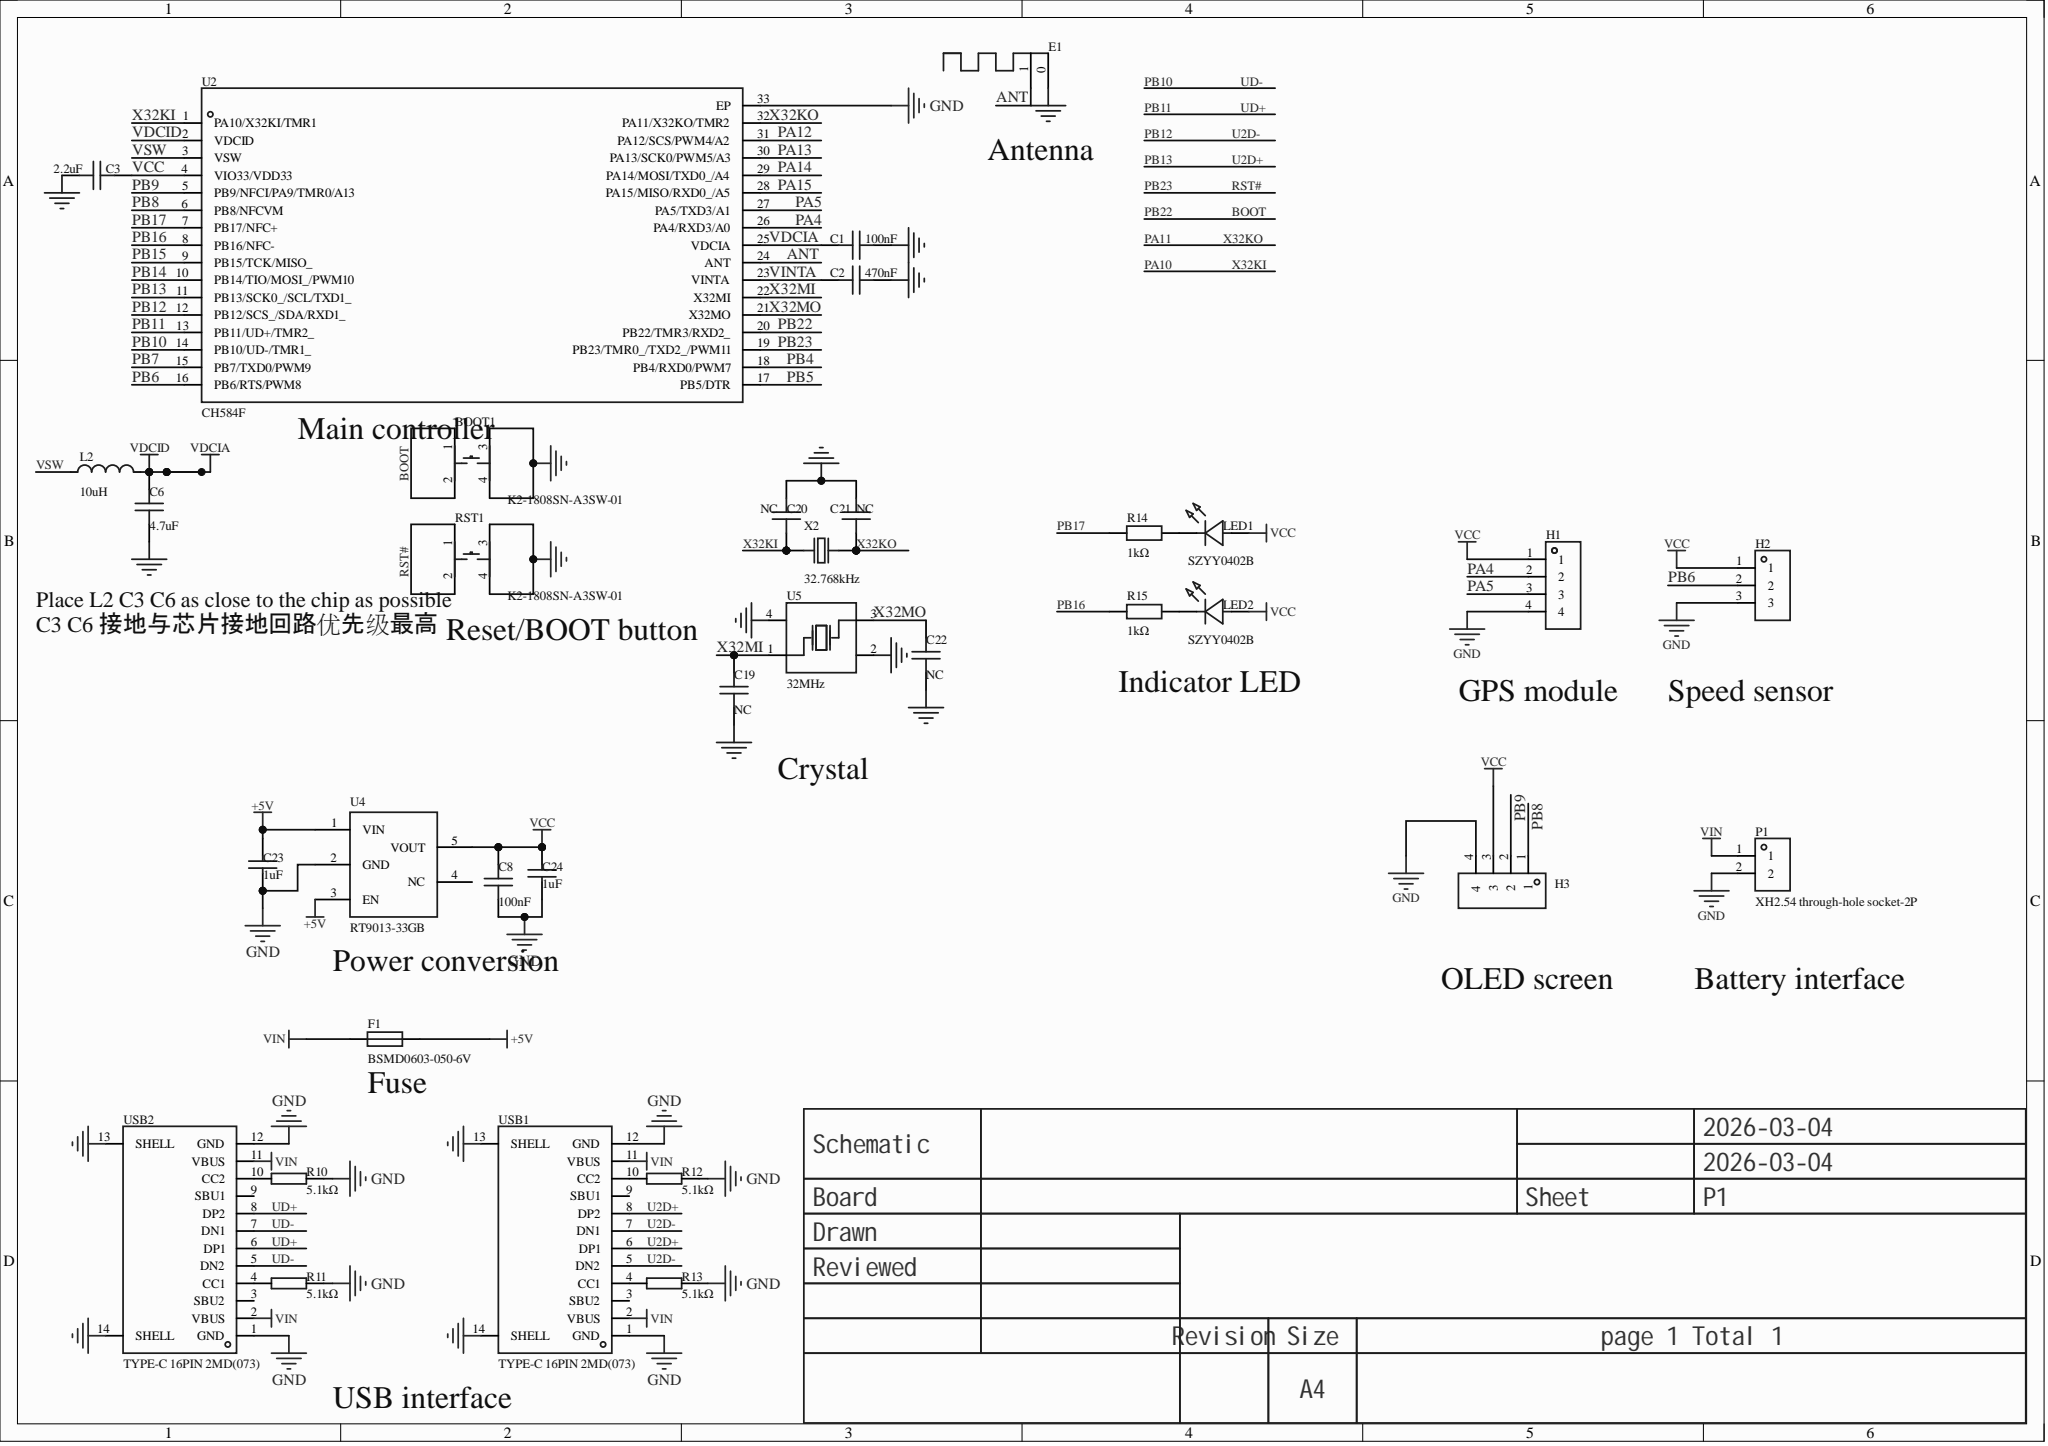Circuit board | Altium Designer | 34 parts | 31 nets
Bill of materials:
Comment,Description,Designator,Footprint,LibRef,Quantity
"K2-1808SN-A3SW-01","","BOOT1, RST1","SW-SMD_4P-L4.2-W3.3-P2.15-LS5.1","K2-1808SN-A3SW-01","2"
"100nF","[NoValue], Capacitance: 100nF; tolerance: ±10%; rated voltage: -; dielectric (temperature coefficient): -;","C1, C8","0402电容（极简封装）","CAP_0402, GCM155R71C104KA55J","2"
"470nF","","C2","0402电容（极简封装）","CAP_0402","1"
"2.2uF","","C3","0402电容（极简封装）","CAP_0402","1"
"4.7uF","","C6","0402电容（极简封装）","CAP_0402","1"
"NC","","C19, C20, C21, C22","0402电容（极简封装）","CAP_0402","4"
"1uF","Capacitance: 1uF; tolerance: ±10%; rated voltage: 16V; temperature coefficient: X5R;","C23, C24","0402电容（极简封装）","EMK105BJ105KV-F","2"
"","","E1","ANT-F-1-2.4G-1.6mmFR4","2.4G天线","1"
"BSMD0603-050-6V","Withstand voltage (Vmax): 6V; max current (Imax): 40A; hold current (Ihold): 500mA; trip current (Itrip): 1A;","F1","F0603","BSMD0603-050-6V","1"
"","","H1, H3","HDR-TH_4P-P2.54-V-F","HDR-F_2.54_1x4P","2"
"","","H2","HDR-TH_3P-P2.54-V-F","HDR-F_2.54_1x3P","1"
"10uH","Inductance: 10uH; tolerance: ±20%; rated current: 1.2A; saturation current (Isat): 1.6A; type: molded inductor;","L2","IND-SMD_L2.5-W2.0","FTC252012S100MBCA","1"
"SZYY0402B","Emitted color: blue; power: -; forward current: 5mA; dominant wavelength: 466nm~469nm; color temperature: -; viewing angle: 120°; packaging: -; operating temperature: -40℃~+85℃;","LED1, LED2","LED0402-RD_BLUE","SZYY0402B","2"
"XH2.54 through-hole socket-2P","","P1","CONN-TH_XH2.54-2P","XH2.54直插座-2P","1"
"5.1kΩ","Resistor type: thick-film resistor; resistance: 1kΩ; tolerance: ±1%; power: 62.5mW; max working voltage: 50V; temperature coefficient: ±100ppm/?;","R10, R11, R12, R13","R0402","0402WGF1001TCE","4"
"1kΩ","Resistor type: thick-film resistor; resistance: 1kΩ; tolerance: ±1%; power: 100mW; max working voltage: 75V; temperature coefficient: ±100ppm/?;","R14, R15","R0603","0603WAF1001T5E","2"
"CH584F","CH585 is a RISC-V MCU/SoC with integrated BLE wireless communication and high-speed USB and NFC. It integrates a 2Mbps low-power Bluetooth BLE communication module, a USB full-speed controller and transceiver, a USB high-speed controller and transceiver (480Mbps), an NFC near-field communication wireless interface, a segment LCD driver module, an LED matrix interface, 2 SPI, 4 UART, 14-channel ADC, touch-key detection module and other rich peripheral resources.","U2","QFN-32_L4.0-W4.0-P0.40-TL-EP2.7","CH584F","1"
"RT9013-33GB","Output type: fixed; output polarity: positive; output channels: 1; max input voltage: 5.5V; output voltage: 3.3V; dropout: 400mV@(500mA); quiescent (ground) current: -; output current: 500mA; PSRR: 50dB@(10kHz); noise: -; features: -;","U4","SOT-23-5_L3.0-W1.7-P0.95-LS2.8-BR","RT9013-33GB","1"
"32MHz","Crystal type: SMD crystal; frequency: 32MHz; frequency deviation at room temperature: ±10ppm; load capacitance: 12pF; frequency stability: ±20ppm;","U5","CRYSTAL-SMD_4P-L2.0-W1.6-BL-2","XL7EL89COI-111YLC-32M","1"
"TYPE-C 16PIN 2MD(073)","Connector type: Type-C; protocol standard: USB 3.1; gender: female; mounting: horizontal SMD; contacts: 16P; ports: 1; rated current - power: 3A; operating temperature: -25℃~+85℃;","USB1, USB2","USB-C-SMD_TYPE-C-6PIN-2MD-073","TYPE-C 16PIN 2MD(073)","2"
"32.768kHz","Crystal type: SMD crystal; frequency: 32.768kHz; frequency deviation at room temperature: ±20ppm; load capacitance: 12.5pF;","X2","FC-135R_L3.2-W1.5","Q13FC13500004_C32346","1"
Netlist (Protel format):
[
BOOT1
SW-SMD_4P-L4.2-W3.3-P2.15-LS5.1
K2-1808SN-A3SW-01



]
[
C1
0402电容（极简封装）
100nF



]
[
C2
0402电容（极简封装）
470nF



]
[
C3
0402电容（极简封装）
2.2uF



]
[
C6
0402电容（极简封装）
4.7uF



]
[
C8
0402电容（极简封装）
100nF



]
[
C19
0402电容（极简封装）
NC



]
[
C20
0402电容（极简封装）
NC



]
[
C21
0402电容（极简封装）
NC



]
[
C22
0402电容（极简封装）
NC



]
[
C23
0402电容（极简封装）
1uF



]
[
C24
0402电容（极简封装）
1uF



]
[
E1
ANT-F-1-2.4G-1.6mmFR4




]
[
F1
F0603
BSMD0603-050-6V



]
[
H1
HDR-TH_4P-P2.54-V-F




]
[
H2
HDR-TH_3P-P2.54-V-F




]
[
H3
HDR-TH_4P-P2.54-V-F




]
[
L2
IND-SMD_L2.5-W2.0
10uH



]
[
LED1
LED0402-RD_BLUE
SZYY0402B



]
[
LED2
LED0402-RD_BLUE
SZYY0402B



]
[
P1
CONN-TH_XH2.54-2P
XH2.54 through-hole socket-2P



]
[
R10
R0402
5.1kΩ



]
[
R11
R0402
5.1kΩ



]
[
R12
R0402
5.1kΩ



]
[
R13
R0402
5.1kΩ



]
[
R14
R0603
1kΩ



]
[
R15
R0603
1kΩ



]
[
RST1
SW-SMD_4P-L4.2-W3.3-P2.15-LS5.1
K2-1808SN-A3SW-01



]
[
U2
QFN-32_L4.0-W4.0-P0.40-TL-EP2.7
CH584F



]
[
U4
SOT-23-5_L3.0-W1.7-P0.95-LS2.8-BR
RT9013-33GB



]
[
U5
CRYSTAL-SMD_4P-L2.0-W1.6-BL-2
32MHz



]
[
USB1
USB-C-SMD_TYPE-C-6PIN-2MD-073
TYPE-C 16PIN 2MD(073)



]
[
USB2
USB-C-SMD_TYPE-C-6PIN-2MD-073
TYPE-C 16PIN 2MD(073)



]
[
X2
FC-135R_L3.2-W1.5
32.768kHz



]
(
X32MO
C22-2
U2-21
U5-3
)
(
X32MI
C19-2
U2-22
U5-1
)
(
VSW
L2-2
U2-3
)
(
VINTA
C2-1
U2-23
)
(
VIN
F1-1
P1-1
USB1-2
USB1-11
USB2-2
USB2-11
)
(
VDCIA
C1-1
C6-2
L2-1
U2-2
U2-25
)
(
VCC
C3-1
C8-2
C24-2
H1-1
H2-1
H3-3
LED1-2
LED2-2
U2-4
U4-5
)
(
PB23
RST1-1
RST1-2
U2-19
)
(
PB17
R14-1
U2-7
)
(
PB16
R15-1
U2-8
)
(
PB13
U2-11
USB1-6
USB1-8
)
(
PB12
U2-12
USB1-5
USB1-7
)
(
PB11
U2-13
USB2-6
USB2-8
)
(
PB10
U2-14
USB2-5
USB2-7
)
(
PB9
H3-2
U2-5
)
(
PB8
H3-1
U2-6
)
(
PB6
H2-2
U2-16
)
(
PA11
C21-1
U2-32
X2-2
)
(
PA10
C20-1
U2-1
X2-1
)
(
PA5
H1-3
U2-27
)
(
PA4
H1-2
U2-26
)
(
NetR13_2
R13-2
USB1-4
)
(
NetR12_2
R12-2
USB1-10
)
(
NetR11_2
R11-2
USB2-4
)
(
NetR10_2
R10-2
USB2-10
)
(
NetLED2_1
LED2-1
R15-2
)
(
NetLED1_1
LED1-1
R14-2
)
(
GND
BOOT1-3
BOOT1-4
C1-2
C2-2
C3-2
C6-1
C8-1
C19-1
C20-2
C21-2
C22-1
C23-1
C24-1
E1-0
H1-4
H2-3
H3-4
P1-2
R10-1
R11-1
R12-1
R13-1
RST1-3
RST1-4
U2-33
U4-2
U5-2
U5-4
USB1-1
USB1-12
USB1-13
USB1-14
USB2-1
USB2-12
USB2-13
USB2-14
)
(
BOOT
BOOT1-1
BOOT1-2
U2-20
)
(
ANT
E1-1
U2-24
)
(
+5V
C23-2
F1-2
U4-1
U4-3
)